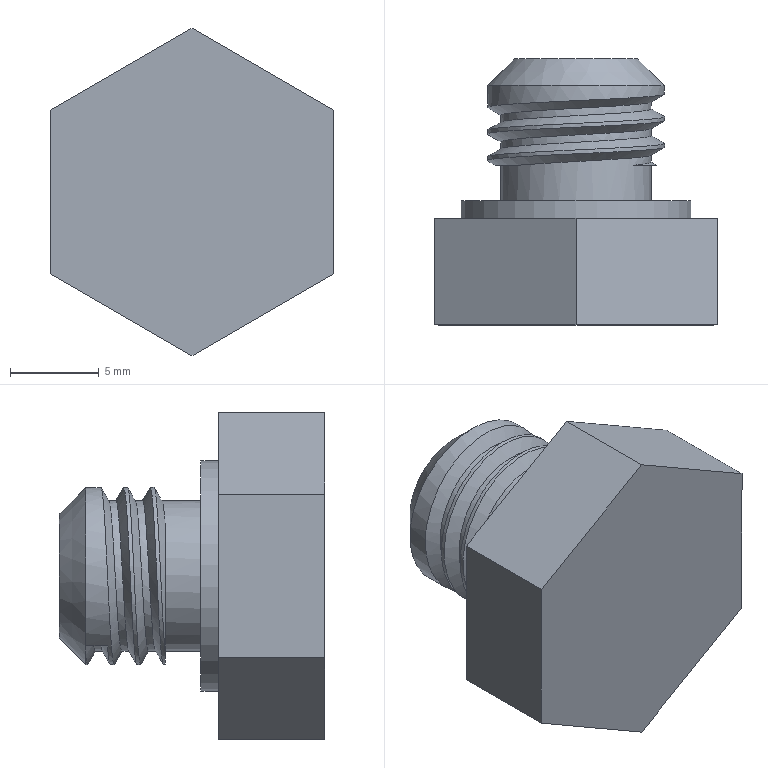Part | NX | features DATUM_CSYS 3, SKETCH 2, EXTRUDE 1, SWP104 1, THREADS 1 | 1 solid | 21 faces | box 16 x 15 x 18.475 mm | volume 1967 mm3 | plane 12 | cylinder 6 | spline 2 | cone 1 | commonest cylinder face diameters 8.5 x4 10 x1 13 x1
STEP:
#1=CARTESIAN_POINT('',(8.,0.,4.619));
#2=VERTEX_POINT('',#1);
#3=CARTESIAN_POINT('',(0.,0.,9.238));
#4=VERTEX_POINT('',#3);
#5=CARTESIAN_POINT('',(8.,0.,4.619));
#6=DIRECTION('',(-0.866,0.,0.5));
#7=VECTOR('',#6,1000.);
#8=LINE('',#5,#7);
#9=EDGE_CURVE('',#2,#4,#8,.T.);
#10=ORIENTED_EDGE('',*,*,#9,.T.);
#11=CARTESIAN_POINT('',(0.,-6.,9.238));
#12=VERTEX_POINT('',#11);
#13=CARTESIAN_POINT('',(0.,-6.,9.238));
#14=DIRECTION('',(0.,1.,0.));
#15=VECTOR('',#14,1000.);
#16=LINE('',#13,#15);
#17=EDGE_CURVE('',#12,#4,#16,.T.);
#18=ORIENTED_EDGE('',*,*,#17,.F.);
#19=CARTESIAN_POINT('',(8.,-6.,4.619));
#20=VERTEX_POINT('',#19);
#21=CARTESIAN_POINT('',(8.,-6.,4.619));
#22=DIRECTION('',(-0.866,0.,0.5));
#23=VECTOR('',#22,1000.);
#24=LINE('',#21,#23);
#25=EDGE_CURVE('',#20,#12,#24,.T.);
#26=ORIENTED_EDGE('',*,*,#25,.F.);
#27=CARTESIAN_POINT('',(8.,-6.,4.619));
#28=DIRECTION('',(0.,1.,0.));
#29=VECTOR('',#28,1000.);
#30=LINE('',#27,#29);
#31=EDGE_CURVE('',#20,#2,#30,.T.);
#32=ORIENTED_EDGE('',*,*,#31,.T.);
#33=EDGE_LOOP('',(#10,#18,#26,#32));
#34=FACE_BOUND('',#33,.T.);
#35=CARTESIAN_POINT('',(8.,-6.,4.619));
#36=DIRECTION('',(-0.5,0.,-0.866));
#37=DIRECTION('',(-0.866,0.,0.5));
#38=AXIS2_PLACEMENT_3D('',#35,#36,#37);
#39=PLANE('',#38);
#40=ADVANCED_FACE('',(#34),#39,.F.);
#41=CARTESIAN_POINT('',(-8.,0.,4.619));
#42=VERTEX_POINT('',#41);
#43=CARTESIAN_POINT('',(0.,0.,9.238));
#44=DIRECTION('',(-0.866,0.,-0.5));
#45=VECTOR('',#44,1000.);
#46=LINE('',#43,#45);
#47=EDGE_CURVE('',#4,#42,#46,.T.);
#48=ORIENTED_EDGE('',*,*,#47,.T.);
#49=CARTESIAN_POINT('',(-8.,-6.,4.619));
#50=VERTEX_POINT('',#49);
#51=CARTESIAN_POINT('',(-8.,-6.,4.619));
#52=DIRECTION('',(0.,1.,0.));
#53=VECTOR('',#52,1000.);
#54=LINE('',#51,#53);
#55=EDGE_CURVE('',#50,#42,#54,.T.);
#56=ORIENTED_EDGE('',*,*,#55,.F.);
#57=CARTESIAN_POINT('',(0.,-6.,9.238));
#58=DIRECTION('',(-0.866,0.,-0.5));
#59=VECTOR('',#58,1000.);
#60=LINE('',#57,#59);
#61=EDGE_CURVE('',#12,#50,#60,.T.);
#62=ORIENTED_EDGE('',*,*,#61,.F.);
#63=ORIENTED_EDGE('',*,*,#17,.T.);
#64=EDGE_LOOP('',(#48,#56,#62,#63));
#65=FACE_BOUND('',#64,.T.);
#66=CARTESIAN_POINT('',(0.,-6.,9.238));
#67=DIRECTION('',(0.5,0.,-0.866));
#68=DIRECTION('',(-0.866,0.,-0.5));
#69=AXIS2_PLACEMENT_3D('',#66,#67,#68);
#70=PLANE('',#69);
#71=ADVANCED_FACE('',(#65),#70,.F.);
#72=CARTESIAN_POINT('',(-8.,0.,-4.619));
#73=VERTEX_POINT('',#72);
#74=CARTESIAN_POINT('',(-8.,0.,4.619));
#75=DIRECTION('',(0.,0.,-1.));
#76=VECTOR('',#75,1000.);
#77=LINE('',#74,#76);
#78=EDGE_CURVE('',#42,#73,#77,.T.);
#79=ORIENTED_EDGE('',*,*,#78,.T.);
#80=CARTESIAN_POINT('',(-8.,-6.,-4.619));
#81=VERTEX_POINT('',#80);
#82=CARTESIAN_POINT('',(-8.,-6.,-4.619));
#83=DIRECTION('',(0.,1.,0.));
#84=VECTOR('',#83,1000.);
#85=LINE('',#82,#84);
#86=EDGE_CURVE('',#81,#73,#85,.T.);
#87=ORIENTED_EDGE('',*,*,#86,.F.);
#88=CARTESIAN_POINT('',(-8.,-6.,4.619));
#89=DIRECTION('',(0.,0.,-1.));
#90=VECTOR('',#89,1000.);
#91=LINE('',#88,#90);
#92=EDGE_CURVE('',#50,#81,#91,.T.);
#93=ORIENTED_EDGE('',*,*,#92,.F.);
#94=ORIENTED_EDGE('',*,*,#55,.T.);
#95=EDGE_LOOP('',(#79,#87,#93,#94));
#96=FACE_BOUND('',#95,.T.);
#97=CARTESIAN_POINT('',(-8.,-6.,4.619));
#98=DIRECTION('',(1.,0.,0.));
#99=DIRECTION('',(0.,0.,-1.));
#100=AXIS2_PLACEMENT_3D('',#97,#98,#99);
#101=PLANE('',#100);
#102=ADVANCED_FACE('',(#96),#101,.F.);
#103=CARTESIAN_POINT('',(0.,0.,-9.238));
#104=VERTEX_POINT('',#103);
#105=CARTESIAN_POINT('',(-8.,0.,-4.619));
#106=DIRECTION('',(0.866,0.,-0.5));
#107=VECTOR('',#106,1000.);
#108=LINE('',#105,#107);
#109=EDGE_CURVE('',#73,#104,#108,.T.);
#110=ORIENTED_EDGE('',*,*,#109,.T.);
#111=CARTESIAN_POINT('',(0.,-6.,-9.238));
#112=VERTEX_POINT('',#111);
#113=CARTESIAN_POINT('',(0.,-6.,-9.238));
#114=DIRECTION('',(0.,1.,0.));
#115=VECTOR('',#114,1000.);
#116=LINE('',#113,#115);
#117=EDGE_CURVE('',#112,#104,#116,.T.);
#118=ORIENTED_EDGE('',*,*,#117,.F.);
#119=CARTESIAN_POINT('',(-8.,-6.,-4.619));
#120=DIRECTION('',(0.866,0.,-0.5));
#121=VECTOR('',#120,1000.);
#122=LINE('',#119,#121);
#123=EDGE_CURVE('',#81,#112,#122,.T.);
#124=ORIENTED_EDGE('',*,*,#123,.F.);
#125=ORIENTED_EDGE('',*,*,#86,.T.);
#126=EDGE_LOOP('',(#110,#118,#124,#125));
#127=FACE_BOUND('',#126,.T.);
#128=CARTESIAN_POINT('',(-8.,-6.,-4.619));
#129=DIRECTION('',(0.5,0.,0.866));
#130=DIRECTION('',(0.866,0.,-0.5));
#131=AXIS2_PLACEMENT_3D('',#128,#129,#130);
#132=PLANE('',#131);
#133=ADVANCED_FACE('',(#127),#132,.F.);
#134=CARTESIAN_POINT('',(8.,0.,-4.619));
#135=VERTEX_POINT('',#134);
#136=CARTESIAN_POINT('',(0.,0.,-9.238));
#137=DIRECTION('',(0.866,0.,0.5));
#138=VECTOR('',#137,1000.);
#139=LINE('',#136,#138);
#140=EDGE_CURVE('',#104,#135,#139,.T.);
#141=ORIENTED_EDGE('',*,*,#140,.T.);
#142=CARTESIAN_POINT('',(8.,-6.,-4.619));
#143=VERTEX_POINT('',#142);
#144=CARTESIAN_POINT('',(8.,-6.,-4.619));
#145=DIRECTION('',(0.,1.,0.));
#146=VECTOR('',#145,1000.);
#147=LINE('',#144,#146);
#148=EDGE_CURVE('',#143,#135,#147,.T.);
#149=ORIENTED_EDGE('',*,*,#148,.F.);
#150=CARTESIAN_POINT('',(0.,-6.,-9.238));
#151=DIRECTION('',(0.866,0.,0.5));
#152=VECTOR('',#151,1000.);
#153=LINE('',#150,#152);
#154=EDGE_CURVE('',#112,#143,#153,.T.);
#155=ORIENTED_EDGE('',*,*,#154,.F.);
#156=ORIENTED_EDGE('',*,*,#117,.T.);
#157=EDGE_LOOP('',(#141,#149,#155,#156));
#158=FACE_BOUND('',#157,.T.);
#159=CARTESIAN_POINT('',(0.,-6.,-9.238));
#160=DIRECTION('',(-0.5,0.,0.866));
#161=DIRECTION('',(0.866,0.,0.5));
#162=AXIS2_PLACEMENT_3D('',#159,#160,#161);
#163=PLANE('',#162);
#164=ADVANCED_FACE('',(#158),#163,.F.);
#165=CARTESIAN_POINT('',(8.,0.,-4.619));
#166=DIRECTION('',(0.,0.,1.));
#167=VECTOR('',#166,1000.);
#168=LINE('',#165,#167);
#169=EDGE_CURVE('',#135,#2,#168,.T.);
#170=ORIENTED_EDGE('',*,*,#169,.T.);
#171=ORIENTED_EDGE('',*,*,#31,.F.);
#172=CARTESIAN_POINT('',(8.,-6.,-4.619));
#173=DIRECTION('',(0.,0.,1.));
#174=VECTOR('',#173,1000.);
#175=LINE('',#172,#174);
#176=EDGE_CURVE('',#143,#20,#175,.T.);
#177=ORIENTED_EDGE('',*,*,#176,.F.);
#178=ORIENTED_EDGE('',*,*,#148,.T.);
#179=EDGE_LOOP('',(#170,#171,#177,#178));
#180=FACE_BOUND('',#179,.T.);
#181=CARTESIAN_POINT('',(8.,-6.,-4.619));
#182=DIRECTION('',(-1.,0.,0.));
#183=DIRECTION('',(0.,0.,1.));
#184=AXIS2_PLACEMENT_3D('',#181,#182,#183);
#185=PLANE('',#184);
#186=ADVANCED_FACE('',(#180),#185,.F.);
#187=ORIENTED_EDGE('',*,*,#25,.T.);
#188=ORIENTED_EDGE('',*,*,#61,.T.);
#189=ORIENTED_EDGE('',*,*,#92,.T.);
#190=ORIENTED_EDGE('',*,*,#123,.T.);
#191=ORIENTED_EDGE('',*,*,#154,.T.);
#192=ORIENTED_EDGE('',*,*,#176,.T.);
#193=EDGE_LOOP('',(#187,#188,#189,#190,#191,#192));
#194=FACE_BOUND('',#193,.T.);
#195=CARTESIAN_POINT('',(0.,-6.,0.));
#196=DIRECTION('',(0.,-1.,0.));
#197=DIRECTION('',(0.,0.,-1.));
#198=AXIS2_PLACEMENT_3D('',#195,#196,#197);
#199=PLANE('',#198);
#200=ADVANCED_FACE('',(#194),#199,.T.);
#201=CARTESIAN_POINT('',(0.,0.,-6.5));
#202=VERTEX_POINT('',#201);
#203=CARTESIAN_POINT('',(0.,0.,0.));
#204=DIRECTION('',(0.,-1.,0.));
#205=DIRECTION('',(0.,0.,-1.));
#206=AXIS2_PLACEMENT_3D('',#203,#204,#205);
#207=CIRCLE('',#206,6.5);
#208=EDGE_CURVE('',#202,#202,#207,.T.);
#209=ORIENTED_EDGE('',*,*,#208,.T.);
#210=EDGE_LOOP('',(#209));
#211=FACE_BOUND('',#210,.T.);
#212=ORIENTED_EDGE('',*,*,#9,.F.);
#213=ORIENTED_EDGE('',*,*,#169,.F.);
#214=ORIENTED_EDGE('',*,*,#140,.F.);
#215=ORIENTED_EDGE('',*,*,#109,.F.);
#216=ORIENTED_EDGE('',*,*,#78,.F.);
#217=ORIENTED_EDGE('',*,*,#47,.F.);
#218=EDGE_LOOP('',(#212,#213,#214,#215,#216,#217));
#219=FACE_BOUND('',#218,.T.);
#220=CARTESIAN_POINT('',(0.,0.,0.));
#221=DIRECTION('',(0.,-1.,0.));
#222=DIRECTION('',(0.,0.,-1.));
#223=AXIS2_PLACEMENT_3D('',#220,#221,#222);
#224=PLANE('',#223);
#225=ADVANCED_FACE('',(#211,#219),#224,.F.);
#226=CARTESIAN_POINT('',(-2.211,7.5,-4.485));
#227=VERTEX_POINT('',#226);
#228=CARTESIAN_POINT('',(-3.071,7.5,-3.945));
#229=VERTEX_POINT('',#228);
#230=CARTESIAN_POINT('',(0.,7.5,0.));
#231=DIRECTION('',(0.,-1.,0.));
#232=DIRECTION('',(0.,0.,-1.));
#233=AXIS2_PLACEMENT_3D('',#230,#231,#232);
#234=CIRCLE('',#233,5.);
#235=EDGE_CURVE('',#227,#229,#234,.T.);
#236=ORIENTED_EDGE('',*,*,#235,.T.);
#237=CARTESIAN_POINT('',(-3.071,6.267,-3.945));
#238=VERTEX_POINT('',#237);
#239=CARTESIAN_POINT('',(-3.071,0.,-3.945));
#240=DIRECTION('',(0.,-1.,0.));
#241=VECTOR('',#240,1000.);
#242=LINE('',#239,#241);
#243=EDGE_CURVE('',#229,#238,#242,.T.);
#244=ORIENTED_EDGE('',*,*,#243,.T.);
#245=CARTESIAN_POINT('',(2.211,3.,-4.485));
#246=VERTEX_POINT('',#245);
#247=CARTESIAN_POINT('',(-3.071,6.267,-3.945));
#248=CARTESIAN_POINT('',(-1.936,6.198,-4.829));
#249=CARTESIAN_POINT('',(1.08,6.063,-5.537));
#250=CARTESIAN_POINT('',(4.899,5.859,-2.814));
#251=CARTESIAN_POINT('',(5.337,5.655,1.848));
#252=CARTESIAN_POINT('',(2.102,5.45,5.241));
#253=CARTESIAN_POINT('',(-2.572,5.246,5.028));
#254=CARTESIAN_POINT('',(-5.484,5.042,1.351));
#255=CARTESIAN_POINT('',(-4.621,4.838,-3.247));
#256=CARTESIAN_POINT('',(-0.5735,4.634,-5.618));
#257=CARTESIAN_POINT('',(3.859,4.43,-4.123));
#258=CARTESIAN_POINT('',(5.644,4.225,0.2145));
#259=CARTESIAN_POINT('',(3.545,4.021,4.396));
#260=CARTESIAN_POINT('',(-0.9981,3.817,5.559));
#261=CARTESIAN_POINT('',(-4.847,3.613,2.897));
#262=CARTESIAN_POINT('',(-5.367,3.409,-1.763));
#263=CARTESIAN_POINT('',(-2.187,3.204,-5.202));
#264=CARTESIAN_POINT('',(0.9203,3.069,-5.121));
#265=CARTESIAN_POINT('',(2.211,3.,-4.485));
#266=B_SPLINE_CURVE_WITH_KNOTS('',3,(#247,#248,#249,#250,#251,#252,#253,#254,#255,#256,#257,#258,#259,#260,#261,#262,#263,#264,#265),.UNSPECIFIED.,.F.,.F.,(4,1,1,1,1,1,1,1,1,1,1,1,1,1,1,1,4),(0.,0.004261,0.008522,0.01278,0.01704,0.02131,0.02557,0.02983,0.03409,0.03835,0.04261,0.04687,0.05113,0.05539,0.05965,0.06392,0.06818),.UNSPECIFIED.);
#267=EDGE_CURVE('',#238,#246,#266,.T.);
#268=ORIENTED_EDGE('',*,*,#267,.T.);
#269=CARTESIAN_POINT('',(-2.211,3.,-4.485));
#270=VERTEX_POINT('',#269);
#271=CARTESIAN_POINT('',(0.,3.,0.));
#272=DIRECTION('',(0.,-1.,0.));
#273=DIRECTION('',(0.,0.,-1.));
#274=AXIS2_PLACEMENT_3D('',#271,#272,#273);
#275=CIRCLE('',#274,5.);
#276=EDGE_CURVE('',#270,#246,#275,.T.);
#277=ORIENTED_EDGE('',*,*,#276,.F.);
#278=CARTESIAN_POINT('',(-2.211,3.,-4.485));
#279=CARTESIAN_POINT('',(-3.1,3.048,-4.046));
#280=CARTESIAN_POINT('',(-4.582,3.14,-2.654));
#281=CARTESIAN_POINT('',(-5.288,3.281,0.3466));
#282=CARTESIAN_POINT('',(-4.201,3.422,3.226));
#283=CARTESIAN_POINT('',(-1.704,3.562,5.015));
#284=CARTESIAN_POINT('',(1.368,3.703,5.118));
#285=CARTESIAN_POINT('',(3.983,3.844,3.494));
#286=CARTESIAN_POINT('',(5.252,3.985,0.6902));
#287=CARTESIAN_POINT('',(4.752,4.125,-2.34));
#288=CARTESIAN_POINT('',(2.652,4.266,-4.586));
#289=CARTESIAN_POINT('',(-0.3453,4.406,-5.287));
#290=CARTESIAN_POINT('',(-3.225,4.547,-4.202));
#291=CARTESIAN_POINT('',(-5.015,4.687,-1.706));
#292=CARTESIAN_POINT('',(-5.118,4.828,1.367));
#293=CARTESIAN_POINT('',(-3.495,4.969,3.982));
#294=CARTESIAN_POINT('',(-0.6915,5.11,5.252));
#295=CARTESIAN_POINT('',(2.338,5.25,4.753));
#296=CARTESIAN_POINT('',(4.586,5.391,2.653));
#297=CARTESIAN_POINT('',(5.287,5.531,-0.3446));
#298=CARTESIAN_POINT('',(4.203,5.672,-3.224));
#299=CARTESIAN_POINT('',(1.708,5.812,-5.014));
#300=CARTESIAN_POINT('',(-1.367,5.953,-5.119));
#301=CARTESIAN_POINT('',(-3.982,6.094,-3.495));
#302=CARTESIAN_POINT('',(-5.251,6.234,-0.6931));
#303=CARTESIAN_POINT('',(-4.754,6.375,2.337));
#304=CARTESIAN_POINT('',(-2.654,6.516,4.586));
#305=CARTESIAN_POINT('',(0.3439,6.656,5.287));
#306=CARTESIAN_POINT('',(3.223,6.797,4.204));
#307=CARTESIAN_POINT('',(5.014,6.937,1.71));
#308=CARTESIAN_POINT('',(5.119,7.078,-1.366));
#309=CARTESIAN_POINT('',(3.496,7.218,-3.982));
#310=CARTESIAN_POINT('',(0.6934,7.36,-5.25));
#311=CARTESIAN_POINT('',(-1.322,7.452,-4.923));
#312=CARTESIAN_POINT('',(-2.211,7.5,-4.485));
#313=B_SPLINE_CURVE_WITH_KNOTS('',3,(#278,#279,#280,#281,#282,#283,#284,#285,#286,#287,#288,#289,#290,#291,#292,#293,#294,#295,#296,#297,#298,#299,#300,#301,#302,#303,#304,#305,#306,#307,#308,#309,#310,#311,#312),.UNSPECIFIED.,.F.,.F.,(4,1,1,1,1,1,1,1,1,1,1,1,1,1,1,1,1,1,1,1,1,1,1,1,1,1,1,1,1,1,1,1,4),(0.,0.002934,0.005869,0.008803,0.01174,0.01467,0.01761,0.02054,0.02348,0.02641,0.02934,0.03228,0.03521,0.03815,0.04108,0.04402,0.04695,0.04989,0.05282,0.05576,0.05869,0.06162,0.06456,0.06749,0.07043,0.07336,0.0763,0.07923,0.08217,0.0851,0.08803,0.09097,0.0939),.UNSPECIFIED.);
#314=EDGE_CURVE('',#270,#227,#313,.T.);
#315=ORIENTED_EDGE('',*,*,#314,.T.);
#316=EDGE_LOOP('',(#236,#244,#268,#277,#315));
#317=FACE_BOUND('',#316,.T.);
#318=CARTESIAN_POINT('',(0.,0.,0.));
#319=DIRECTION('',(0.,-1.,0.));
#320=DIRECTION('',(0.,0.,-1.));
#321=AXIS2_PLACEMENT_3D('',#318,#319,#320);
#322=CYLINDRICAL_SURFACE('',#321,5.);
#323=ADVANCED_FACE('',(#317),#322,.T.);
#324=ORIENTED_EDGE('',*,*,#276,.T.);
#325=CARTESIAN_POINT('',(3.248,3.,2.741));
#326=VERTEX_POINT('',#325);
#327=CARTESIAN_POINT('',(2.211,3.,-4.485));
#328=CARTESIAN_POINT('',(3.421,3.,-3.758));
#329=CARTESIAN_POINT('',(5.166,3.,-1.231));
#330=CARTESIAN_POINT('',(4.262,3.,1.752));
#331=CARTESIAN_POINT('',(3.248,3.,2.741));
#332=B_SPLINE_CURVE_WITH_KNOTS('',3,(#327,#328,#329,#330,#331),.UNSPECIFIED.,.F.,.F.,(4,1,4),(0.0001186,0.004308,0.008497),.UNSPECIFIED.);
#333=EDGE_CURVE('',#246,#326,#332,.T.);
#334=ORIENTED_EDGE('',*,*,#333,.T.);
#335=CARTESIAN_POINT('',(-3.248,3.,2.741));
#336=VERTEX_POINT('',#335);
#337=CARTESIAN_POINT('',(0.,3.,0.));
#338=DIRECTION('',(0.,-1.,0.));
#339=DIRECTION('',(0.,0.,-1.));
#340=AXIS2_PLACEMENT_3D('',#337,#338,#339);
#341=CIRCLE('',#340,4.25);
#342=EDGE_CURVE('',#336,#326,#341,.T.);
#343=ORIENTED_EDGE('',*,*,#342,.F.);
#344=CARTESIAN_POINT('',(-3.248,3.,2.741));
#345=CARTESIAN_POINT('',(-4.26,3.,1.753));
#346=CARTESIAN_POINT('',(-5.168,3.,-1.228));
#347=CARTESIAN_POINT('',(-3.42,3.,-3.758));
#348=CARTESIAN_POINT('',(-2.211,3.,-4.485));
#349=B_SPLINE_CURVE_WITH_KNOTS('',3,(#344,#345,#346,#347,#348),.UNSPECIFIED.,.F.,.F.,(4,1,4),(0.00004919,0.004257,0.008466),.UNSPECIFIED.);
#350=EDGE_CURVE('',#336,#270,#349,.T.);
#351=ORIENTED_EDGE('',*,*,#350,.T.);
#352=EDGE_LOOP('',(#324,#334,#343,#351));
#353=FACE_BOUND('',#352,.T.);
#354=CARTESIAN_POINT('',(0.,3.,5.));
#355=DIRECTION('',(0.,1.,0.));
#356=DIRECTION('',(0.,0.,1.));
#357=AXIS2_PLACEMENT_3D('',#354,#355,#356);
#358=PLANE('',#357);
#359=ADVANCED_FACE('',(#353),#358,.F.);
#360=CARTESIAN_POINT('',(0.,1.,-4.25));
#361=VERTEX_POINT('',#360);
#362=CARTESIAN_POINT('',(0.,1.,0.));
#363=DIRECTION('',(0.,-1.,0.));
#364=DIRECTION('',(0.,0.,-1.));
#365=AXIS2_PLACEMENT_3D('',#362,#363,#364);
#366=CIRCLE('',#365,4.25);
#367=EDGE_CURVE('',#361,#361,#366,.T.);
#368=ORIENTED_EDGE('',*,*,#367,.F.);
#369=EDGE_LOOP('',(#368));
#370=FACE_BOUND('',#369,.T.);
#371=ORIENTED_EDGE('',*,*,#342,.T.);
#372=CARTESIAN_POINT('',(-2.611,6.7,-3.354));
#373=VERTEX_POINT('',#372);
#374=CARTESIAN_POINT('',(-2.611,6.7,-3.354));
#375=CARTESIAN_POINT('',(-1.518,6.622,-4.205));
#376=CARTESIAN_POINT('',(1.501,6.469,-4.728));
#377=CARTESIAN_POINT('',(4.755,6.238,-1.443));
#378=CARTESIAN_POINT('',(3.881,6.006,3.102));
#379=CARTESIAN_POINT('',(-0.3584,5.775,4.955));
#380=CARTESIAN_POINT('',(-4.288,5.544,2.51));
#381=CARTESIAN_POINT('',(-4.497,5.313,-2.113));
#382=CARTESIAN_POINT('',(-0.8052,5.081,-4.902));
#383=CARTESIAN_POINT('',(3.584,4.85,-3.44));
#384=CARTESIAN_POINT('',(4.865,4.619,1.003));
#385=CARTESIAN_POINT('',(1.93,4.388,4.578));
#386=CARTESIAN_POINT('',(-2.68,4.156,4.184));
#387=CARTESIAN_POINT('',(-4.966,3.925,0.1601));
#388=CARTESIAN_POINT('',(-2.944,3.694,-4.002));
#389=CARTESIAN_POINT('',(1.634,3.463,-4.694));
#390=CARTESIAN_POINT('',(4.786,3.231,-1.306));
#391=CARTESIAN_POINT('',(4.14,3.077,1.685));
#392=CARTESIAN_POINT('',(3.248,3.,2.741));
#393=B_SPLINE_CURVE_WITH_KNOTS('',3,(#374,#375,#376,#377,#378,#379,#380,#381,#382,#383,#384,#385,#386,#387,#388,#389,#390,#391,#392),.UNSPECIFIED.,.F.,.F.,(4,1,1,1,1,1,1,1,1,1,1,1,1,1,1,1,4),(0.,0.004122,0.008243,0.01236,0.01649,0.02061,0.02473,0.02885,0.03297,0.03709,0.04122,0.04534,0.04946,0.05358,0.0577,0.06182,0.06595),.UNSPECIFIED.);
#394=EDGE_CURVE('',#373,#326,#393,.T.);
#395=ORIENTED_EDGE('',*,*,#394,.F.);
#396=CARTESIAN_POINT('',(-2.611,7.116,-3.354));
#397=VERTEX_POINT('',#396);
#398=CARTESIAN_POINT('',(-2.611,2.25,-3.354));
#399=DIRECTION('',(0.,1.,0.));
#400=VECTOR('',#399,1000.);
#401=LINE('',#398,#400);
#402=EDGE_CURVE('',#397,#373,#401,.F.);
#403=ORIENTED_EDGE('',*,*,#402,.F.);
#404=CARTESIAN_POINT('',(-3.248,3.,2.741));
#405=CARTESIAN_POINT('',(-2.259,3.086,3.912));
#406=CARTESIAN_POINT('',(1.06,3.258,5.037));
#407=CARTESIAN_POINT('',(4.948,3.515,1.451));
#408=CARTESIAN_POINT('',(3.62,3.772,-3.669));
#409=CARTESIAN_POINT('',(-1.514,4.029,-4.926));
#410=CARTESIAN_POINT('',(-5.057,4.286,-1.));
#411=CARTESIAN_POINT('',(-3.274,4.543,3.982));
#412=CARTESIAN_POINT('',(1.957,4.801,4.768));
#413=CARTESIAN_POINT('',(5.126,5.058,0.5354));
#414=CARTESIAN_POINT('',(2.901,5.315,-4.26));
#415=CARTESIAN_POINT('',(-2.377,5.572,-4.573));
#416=CARTESIAN_POINT('',(-5.155,5.829,-0.07114));
#417=CARTESIAN_POINT('',(-2.501,6.087,4.507));
#418=CARTESIAN_POINT('',(2.783,6.344,4.338));
#419=CARTESIAN_POINT('',(5.141,6.601,-0.3979));
#420=CARTESIAN_POINT('',(2.078,6.858,-4.706));
#421=CARTESIAN_POINT('',(-1.395,7.029,-4.3));
#422=CARTESIAN_POINT('',(-2.611,7.116,-3.354));
#423=B_SPLINE_CURVE_WITH_KNOTS('',3,(#404,#405,#406,#407,#408,#409,#410,#411,#412,#413,#414,#415,#416,#417,#418,#419,#420,#421,#422),.UNSPECIFIED.,.F.,.F.,(4,1,1,1,1,1,1,1,1,1,1,1,1,1,1,1,4),(0.009664,0.01425,0.01883,0.02342,0.028,0.03259,0.03717,0.04175,0.04634,0.05092,0.05551,0.06009,0.06468,0.06926,0.07384,0.07843,0.08301),.UNSPECIFIED.);
#424=EDGE_CURVE('',#336,#397,#423,.T.);
#425=ORIENTED_EDGE('',*,*,#424,.F.);
#426=EDGE_LOOP('',(#371,#395,#403,#425));
#427=FACE_BOUND('',#426,.T.);
#428=CARTESIAN_POINT('',(0.,0.,0.));
#429=DIRECTION('',(0.,-1.,0.));
#430=DIRECTION('',(0.,0.,-1.));
#431=AXIS2_PLACEMENT_3D('',#428,#429,#430);
#432=CYLINDRICAL_SURFACE('',#431,4.25);
#433=ADVANCED_FACE('',(#370,#427),#432,.T.);
#434=CARTESIAN_POINT('',(0.,1.,-6.5));
#435=VERTEX_POINT('',#434);
#436=CARTESIAN_POINT('',(0.,1.,0.));
#437=DIRECTION('',(0.,-1.,0.));
#438=DIRECTION('',(0.,0.,-1.));
#439=AXIS2_PLACEMENT_3D('',#436,#437,#438);
#440=CIRCLE('',#439,6.5);
#441=EDGE_CURVE('',#435,#435,#440,.T.);
#442=ORIENTED_EDGE('',*,*,#441,.F.);
#443=EDGE_LOOP('',(#442));
#444=FACE_BOUND('',#443,.T.);
#445=ORIENTED_EDGE('',*,*,#367,.T.);
#446=EDGE_LOOP('',(#445));
#447=FACE_BOUND('',#446,.T.);
#448=CARTESIAN_POINT('',(0.,1.,4.25));
#449=DIRECTION('',(0.,-1.,0.));
#450=DIRECTION('',(0.,0.,-1.));
#451=AXIS2_PLACEMENT_3D('',#448,#449,#450);
#452=PLANE('',#451);
#453=ADVANCED_FACE('',(#444,#447),#452,.F.);
#454=ORIENTED_EDGE('',*,*,#208,.F.);
#455=EDGE_LOOP('',(#454));
#456=FACE_BOUND('',#455,.T.);
#457=ORIENTED_EDGE('',*,*,#441,.T.);
#458=EDGE_LOOP('',(#457));
#459=FACE_BOUND('',#458,.T.);
#460=CARTESIAN_POINT('',(0.,0.,0.));
#461=DIRECTION('',(0.,-1.,0.));
#462=DIRECTION('',(0.,0.,-1.));
#463=AXIS2_PLACEMENT_3D('',#460,#461,#462);
#464=CYLINDRICAL_SURFACE('',#463,6.5);
#465=ADVANCED_FACE('',(#456,#459),#464,.T.);
#466=CARTESIAN_POINT('',(0.,9.,-3.5));
#467=VERTEX_POINT('',#466);
#468=CARTESIAN_POINT('',(0.,9.,0.));
#469=DIRECTION('',(0.,-1.,0.));
#470=DIRECTION('',(0.,0.,-1.));
#471=AXIS2_PLACEMENT_3D('',#468,#469,#470);
#472=CIRCLE('',#471,3.5);
#473=EDGE_CURVE('',#467,#467,#472,.T.);
#474=ORIENTED_EDGE('',*,*,#473,.F.);
#475=EDGE_LOOP('',(#474));
#476=FACE_BOUND('',#475,.T.);
#477=CARTESIAN_POINT('',(0.,9.,0.));
#478=DIRECTION('',(0.,-1.,0.));
#479=DIRECTION('',(0.,0.,-1.));
#480=AXIS2_PLACEMENT_3D('',#477,#478,#479);
#481=PLANE('',#480);
#482=ADVANCED_FACE('',(#476),#481,.F.);
#483=CARTESIAN_POINT('',(-3.053,7.531,-3.921));
#484=VERTEX_POINT('',#483);
#485=CARTESIAN_POINT('',(-2.211,7.5,-4.485));
#486=CARTESIAN_POINT('',(-2.511,7.51,-4.325));
#487=CARTESIAN_POINT('',(-2.791,7.521,-4.138));
#488=CARTESIAN_POINT('',(-3.053,7.531,-3.921));
#489=B_SPLINE_CURVE_WITH_KNOTS('',3,(#485,#486,#487,#488),.UNSPECIFIED.,.F.,.F.,(4,4),(0.,0.001013),.UNSPECIFIED.);
#490=EDGE_CURVE('',#227,#484,#489,.T.);
#491=ORIENTED_EDGE('',*,*,#490,.T.);
#492=CARTESIAN_POINT('',(0.,12.5,0.));
#493=DIRECTION('',(-0.4344,-0.7071,-0.558));
#494=VECTOR('',#493,1000.);
#495=LINE('',#492,#494);
#496=EDGE_CURVE('',#484,#229,#495,.T.);
#497=ORIENTED_EDGE('',*,*,#496,.T.);
#498=ORIENTED_EDGE('',*,*,#235,.F.);
#499=EDGE_LOOP('',(#491,#497,#498));
#500=FACE_BOUND('',#499,.T.);
#501=ORIENTED_EDGE('',*,*,#473,.T.);
#502=EDGE_LOOP('',(#501));
#503=FACE_BOUND('',#502,.T.);
#504=CARTESIAN_POINT('',(0.,9.,0.));
#505=DIRECTION('',(0.,-1.,0.));
#506=DIRECTION('',(0.,0.,-1.));
#507=AXIS2_PLACEMENT_3D('',#504,#505,#506);
#508=CONICAL_SURFACE('',#507,3.5,0.7854);
#509=ADVANCED_FACE('',(#500,#503),#508,.T.);
#510=ORIENTED_EDGE('',*,*,#496,.F.);
#511=CARTESIAN_POINT('',(-2.459,6.973,-3.158));
#512=CARTESIAN_POINT('',(-3.077,7.554,-3.953));
#513=B_SPLINE_CURVE_WITH_KNOTS('',1,(#511,#512),.UNSPECIFIED.,.F.,.F.,(2,2),(0.,1.),.PIECEWISE_BEZIER_KNOTS.);
#514=EDGE_CURVE('',#397,#484,#513,.T.);
#515=ORIENTED_EDGE('',*,*,#514,.F.);
#516=ORIENTED_EDGE('',*,*,#402,.T.);
#517=CARTESIAN_POINT('',(-3.077,6.262,-3.953));
#518=CARTESIAN_POINT('',(-2.459,6.843,-3.158));
#519=B_SPLINE_CURVE_WITH_KNOTS('',1,(#517,#518),.UNSPECIFIED.,.F.,.F.,(2,2),(0.,1.),.PIECEWISE_BEZIER_KNOTS.);
#520=EDGE_CURVE('',#238,#373,#519,.T.);
#521=ORIENTED_EDGE('',*,*,#520,.F.);
#522=ORIENTED_EDGE('',*,*,#243,.F.);
#523=EDGE_LOOP('',(#510,#515,#516,#521,#522));
#524=FACE_BOUND('',#523,.T.);
#525=CARTESIAN_POINT('',(-3.077,6.908,-3.953));
#526=DIRECTION('',(-0.7891,0.,0.6143));
#527=DIRECTION('',(0.6143,0.,0.7891));
#528=AXIS2_PLACEMENT_3D('',#525,#526,#527);
#529=PLANE('',#528);
#530=ADVANCED_FACE('',(#524),#529,.F.);
#531=ORIENTED_EDGE('',*,*,#520,.T.);
#532=ORIENTED_EDGE('',*,*,#394,.T.);
#533=ORIENTED_EDGE('',*,*,#333,.F.);
#534=ORIENTED_EDGE('',*,*,#267,.F.);
#535=EDGE_LOOP('',(#531,#532,#533,#534));
#536=FACE_BOUND('',#535,.T.);
#537=CARTESIAN_POINT('',(3.508,2.542,3.57));
#538=CARTESIAN_POINT('',(3.519,2.543,3.559));
#539=CARTESIAN_POINT('',(3.994,2.575,3.088));
#540=CARTESIAN_POINT('',(4.744,2.638,1.965));
#541=CARTESIAN_POINT('',(5.135,2.732,0.));
#542=CARTESIAN_POINT('',(4.744,2.825,-1.965));
#543=CARTESIAN_POINT('',(3.631,2.919,-3.631));
#544=CARTESIAN_POINT('',(1.965,3.013,-4.744));
#545=CARTESIAN_POINT('',(0.,3.107,-5.135));
#546=CARTESIAN_POINT('',(-1.965,3.2,-4.744));
#547=CARTESIAN_POINT('',(-3.631,3.294,-3.631));
#548=CARTESIAN_POINT('',(-4.744,3.388,-1.965));
#549=CARTESIAN_POINT('',(-5.135,3.482,0.));
#550=CARTESIAN_POINT('',(-4.744,3.575,1.965));
#551=CARTESIAN_POINT('',(-3.631,3.669,3.631));
#552=CARTESIAN_POINT('',(-1.965,3.763,4.744));
#553=CARTESIAN_POINT('',(0.,3.857,5.135));
#554=CARTESIAN_POINT('',(1.965,3.95,4.744));
#555=CARTESIAN_POINT('',(3.631,4.044,3.631));
#556=CARTESIAN_POINT('',(4.744,4.138,1.965));
#557=CARTESIAN_POINT('',(5.135,4.232,0.));
#558=CARTESIAN_POINT('',(4.744,4.325,-1.965));
#559=CARTESIAN_POINT('',(3.631,4.419,-3.631));
#560=CARTESIAN_POINT('',(1.965,4.513,-4.744));
#561=CARTESIAN_POINT('',(0.,4.607,-5.135));
#562=CARTESIAN_POINT('',(-1.965,4.7,-4.744));
#563=CARTESIAN_POINT('',(-3.631,4.794,-3.631));
#564=CARTESIAN_POINT('',(-4.744,4.888,-1.965));
#565=CARTESIAN_POINT('',(-5.135,4.982,0.));
#566=CARTESIAN_POINT('',(-4.744,5.075,1.965));
#567=CARTESIAN_POINT('',(-3.631,5.169,3.631));
#568=CARTESIAN_POINT('',(-1.965,5.263,4.744));
#569=CARTESIAN_POINT('',(0.,5.357,5.135));
#570=CARTESIAN_POINT('',(1.965,5.45,4.744));
#571=CARTESIAN_POINT('',(3.631,5.544,3.631));
#572=CARTESIAN_POINT('',(4.744,5.638,1.965));
#573=CARTESIAN_POINT('',(5.135,5.732,0.));
#574=CARTESIAN_POINT('',(4.744,5.825,-1.965));
#575=CARTESIAN_POINT('',(3.631,5.919,-3.631));
#576=CARTESIAN_POINT('',(1.965,6.013,-4.744));
#577=CARTESIAN_POINT('',(0.,6.107,-5.135));
#578=CARTESIAN_POINT('',(-1.758,6.19,-4.785));
#579=CARTESIAN_POINT('',(-2.72,6.243,-4.224));
#580=CARTESIAN_POINT('',(-3.074,6.264,-3.949));
#581=CARTESIAN_POINT('',(2.976,2.981,3.028));
#582=CARTESIAN_POINT('',(2.985,2.981,3.019));
#583=CARTESIAN_POINT('',(3.388,3.013,2.619));
#584=CARTESIAN_POINT('',(4.024,3.076,1.667));
#585=CARTESIAN_POINT('',(4.356,3.17,0.));
#586=CARTESIAN_POINT('',(4.024,3.264,-1.667));
#587=CARTESIAN_POINT('',(3.08,3.358,-3.08));
#588=CARTESIAN_POINT('',(1.667,3.451,-4.024));
#589=CARTESIAN_POINT('',(0.,3.545,-4.356));
#590=CARTESIAN_POINT('',(-1.667,3.639,-4.024));
#591=CARTESIAN_POINT('',(-3.08,3.733,-3.08));
#592=CARTESIAN_POINT('',(-4.024,3.826,-1.667));
#593=CARTESIAN_POINT('',(-4.356,3.92,0.));
#594=CARTESIAN_POINT('',(-4.024,4.014,1.667));
#595=CARTESIAN_POINT('',(-3.08,4.108,3.08));
#596=CARTESIAN_POINT('',(-1.667,4.201,4.024));
#597=CARTESIAN_POINT('',(0.,4.295,4.356));
#598=CARTESIAN_POINT('',(1.667,4.389,4.024));
#599=CARTESIAN_POINT('',(3.08,4.483,3.08));
#600=CARTESIAN_POINT('',(4.024,4.576,1.667));
#601=CARTESIAN_POINT('',(4.356,4.67,0.));
#602=CARTESIAN_POINT('',(4.024,4.764,-1.667));
#603=CARTESIAN_POINT('',(3.08,4.858,-3.08));
#604=CARTESIAN_POINT('',(1.667,4.951,-4.024));
#605=CARTESIAN_POINT('',(0.,5.045,-4.356));
#606=CARTESIAN_POINT('',(-1.667,5.139,-4.024));
#607=CARTESIAN_POINT('',(-3.08,5.233,-3.08));
#608=CARTESIAN_POINT('',(-4.024,5.326,-1.667));
#609=CARTESIAN_POINT('',(-4.356,5.42,0.));
#610=CARTESIAN_POINT('',(-4.024,5.514,1.667));
#611=CARTESIAN_POINT('',(-3.08,5.608,3.08));
#612=CARTESIAN_POINT('',(-1.667,5.701,4.024));
#613=CARTESIAN_POINT('',(0.,5.795,4.356));
#614=CARTESIAN_POINT('',(1.667,5.889,4.024));
#615=CARTESIAN_POINT('',(3.08,5.983,3.08));
#616=CARTESIAN_POINT('',(4.024,6.076,1.667));
#617=CARTESIAN_POINT('',(4.356,6.17,0.));
#618=CARTESIAN_POINT('',(4.024,6.264,-1.667));
#619=CARTESIAN_POINT('',(3.08,6.358,-3.08));
#620=CARTESIAN_POINT('',(1.667,6.451,-4.024));
#621=CARTESIAN_POINT('',(0.,6.545,-4.356));
#622=CARTESIAN_POINT('',(-1.492,6.629,-4.059));
#623=CARTESIAN_POINT('',(-2.308,6.682,-3.583));
#624=CARTESIAN_POINT('',(-2.608,6.703,-3.35));
#625=B_SPLINE_SURFACE_WITH_KNOTS('',1,3,((#537,#538,#539,#540,#541,#542,#543,#544,#545,#546,#547,#548,#549,#550,#551,#552,#553,#554,#555,#556,#557,#558,#559,#560,#561,#562,#563,#564,#565,#566,#567,#568,#569,#570,#571,#572,#573,#574,#575,#576,#577,#578,#579,#580),(#581,#582,#583,#584,#585,#586,#587,#588,#589,#590,#591,#592,#593,#594,#595,#596,#597,#598,#599,#600,#601,#602,#603,#604,#605,#606,#607,#608,#609,#610,#611,#612,#613,#614,#615,#616,#617,#618,#619,#620,#621,#622,#623,#624)),.RULED_SURF.,.F.,.F.,.F.,(2,2),(4,1,1,1,1,1,1,1,1,1,1,1,1,1,1,1,1,1,1,1,1,1,1,1,1,1,1,1,1,1,1,1,1,1,1,1,1,1,1,1,1,4),(0.005015,0.7593),(0.2008,0.2013,0.2214,0.2415,0.2617,0.2818,0.3019,0.322,0.3422,0.3623,0.3824,0.4025,0.4227,0.4428,0.4629,0.483,0.5032,0.5233,0.5434,0.5636,0.5837,0.6038,0.6239,0.6441,0.6642,0.6843,0.7044,0.7246,0.7447,0.7648,0.785,0.8051,0.8252,0.8453,0.8655,0.8856,0.9057,0.9258,0.946,0.9661,0.9862,1.),.UNSPECIFIED.);
#626=ADVANCED_FACE('',(#536),#625,.F.);
#627=ORIENTED_EDGE('',*,*,#424,.T.);
#628=ORIENTED_EDGE('',*,*,#514,.T.);
#629=ORIENTED_EDGE('',*,*,#490,.F.);
#630=ORIENTED_EDGE('',*,*,#314,.F.);
#631=ORIENTED_EDGE('',*,*,#350,.F.);
#632=EDGE_LOOP('',(#627,#628,#629,#630,#631));
#633=FACE_BOUND('',#632,.T.);
#634=CARTESIAN_POINT('',(-1.431,2.537,-3.997));
#635=CARTESIAN_POINT('',(-1.496,2.541,-3.974));
#636=CARTESIAN_POINT('',(-2.079,2.576,-3.749));
#637=CARTESIAN_POINT('',(-3.08,2.642,-3.08));
#638=CARTESIAN_POINT('',(-4.024,2.736,-1.667));
#639=CARTESIAN_POINT('',(-4.356,2.83,0.));
#640=CARTESIAN_POINT('',(-4.024,2.924,1.667));
#641=CARTESIAN_POINT('',(-3.08,3.017,3.08));
#642=CARTESIAN_POINT('',(-1.667,3.111,4.024));
#643=CARTESIAN_POINT('',(0.,3.205,4.356));
#644=CARTESIAN_POINT('',(1.667,3.299,4.024));
#645=CARTESIAN_POINT('',(3.08,3.392,3.08));
#646=CARTESIAN_POINT('',(4.024,3.486,1.667));
#647=CARTESIAN_POINT('',(4.356,3.58,0.));
#648=CARTESIAN_POINT('',(4.024,3.674,-1.667));
#649=CARTESIAN_POINT('',(3.08,3.767,-3.08));
#650=CARTESIAN_POINT('',(1.667,3.861,-4.024));
#651=CARTESIAN_POINT('',(0.,3.955,-4.356));
#652=CARTESIAN_POINT('',(-1.667,4.049,-4.024));
#653=CARTESIAN_POINT('',(-3.08,4.142,-3.08));
#654=CARTESIAN_POINT('',(-4.024,4.236,-1.667));
#655=CARTESIAN_POINT('',(-4.356,4.33,0.));
#656=CARTESIAN_POINT('',(-4.024,4.424,1.667));
#657=CARTESIAN_POINT('',(-3.08,4.517,3.08));
#658=CARTESIAN_POINT('',(-1.667,4.611,4.024));
#659=CARTESIAN_POINT('',(0.,4.705,4.356));
#660=CARTESIAN_POINT('',(1.667,4.799,4.024));
#661=CARTESIAN_POINT('',(3.08,4.892,3.08));
#662=CARTESIAN_POINT('',(4.024,4.986,1.667));
#663=CARTESIAN_POINT('',(4.356,5.08,0.));
#664=CARTESIAN_POINT('',(4.024,5.174,-1.667));
#665=CARTESIAN_POINT('',(3.08,5.267,-3.08));
#666=CARTESIAN_POINT('',(1.667,5.361,-4.024));
#667=CARTESIAN_POINT('',(0.,5.455,-4.356));
#668=CARTESIAN_POINT('',(-1.667,5.549,-4.024));
#669=CARTESIAN_POINT('',(-3.08,5.642,-3.08));
#670=CARTESIAN_POINT('',(-4.024,5.736,-1.667));
#671=CARTESIAN_POINT('',(-4.356,5.83,0.));
#672=CARTESIAN_POINT('',(-4.024,5.924,1.667));
#673=CARTESIAN_POINT('',(-3.08,6.017,3.08));
#674=CARTESIAN_POINT('',(-1.667,6.111,4.024));
#675=CARTESIAN_POINT('',(0.,6.205,4.356));
#676=CARTESIAN_POINT('',(1.667,6.299,4.024));
#677=CARTESIAN_POINT('',(3.08,6.392,3.08));
#678=CARTESIAN_POINT('',(4.024,6.486,1.667));
#679=CARTESIAN_POINT('',(4.356,6.58,0.));
#680=CARTESIAN_POINT('',(4.024,6.674,-1.667));
#681=CARTESIAN_POINT('',(3.08,6.767,-3.08));
#682=CARTESIAN_POINT('',(1.667,6.861,-4.024));
#683=CARTESIAN_POINT('',(0.,6.955,-4.356));
#684=CARTESIAN_POINT('',(-1.492,7.039,-4.059));
#685=CARTESIAN_POINT('',(-2.308,7.091,-3.583));
#686=CARTESIAN_POINT('',(-2.608,7.113,-3.35));
#687=CARTESIAN_POINT('',(-1.687,2.975,-4.712));
#688=CARTESIAN_POINT('',(-1.764,2.979,-4.685));
#689=CARTESIAN_POINT('',(-2.451,3.015,-4.419));
#690=CARTESIAN_POINT('',(-3.631,3.081,-3.631));
#691=CARTESIAN_POINT('',(-4.744,3.175,-1.965));
#692=CARTESIAN_POINT('',(-5.135,3.268,0.));
#693=CARTESIAN_POINT('',(-4.744,3.362,1.965));
#694=CARTESIAN_POINT('',(-3.631,3.456,3.631));
#695=CARTESIAN_POINT('',(-1.965,3.55,4.744));
#696=CARTESIAN_POINT('',(0.,3.643,5.135));
#697=CARTESIAN_POINT('',(1.965,3.737,4.744));
#698=CARTESIAN_POINT('',(3.631,3.831,3.631));
#699=CARTESIAN_POINT('',(4.744,3.925,1.965));
#700=CARTESIAN_POINT('',(5.135,4.018,0.));
#701=CARTESIAN_POINT('',(4.744,4.112,-1.965));
#702=CARTESIAN_POINT('',(3.631,4.206,-3.631));
#703=CARTESIAN_POINT('',(1.965,4.3,-4.744));
#704=CARTESIAN_POINT('',(0.,4.393,-5.135));
#705=CARTESIAN_POINT('',(-1.965,4.487,-4.744));
#706=CARTESIAN_POINT('',(-3.631,4.581,-3.631));
#707=CARTESIAN_POINT('',(-4.744,4.675,-1.965));
#708=CARTESIAN_POINT('',(-5.135,4.768,0.));
#709=CARTESIAN_POINT('',(-4.744,4.862,1.965));
#710=CARTESIAN_POINT('',(-3.631,4.956,3.631));
#711=CARTESIAN_POINT('',(-1.965,5.05,4.744));
#712=CARTESIAN_POINT('',(0.,5.143,5.135));
#713=CARTESIAN_POINT('',(1.965,5.237,4.744));
#714=CARTESIAN_POINT('',(3.631,5.331,3.631));
#715=CARTESIAN_POINT('',(4.744,5.425,1.965));
#716=CARTESIAN_POINT('',(5.135,5.518,0.));
#717=CARTESIAN_POINT('',(4.744,5.612,-1.965));
#718=CARTESIAN_POINT('',(3.631,5.706,-3.631));
#719=CARTESIAN_POINT('',(1.965,5.8,-4.744));
#720=CARTESIAN_POINT('',(0.,5.893,-5.135));
#721=CARTESIAN_POINT('',(-1.965,5.987,-4.744));
#722=CARTESIAN_POINT('',(-3.631,6.081,-3.631));
#723=CARTESIAN_POINT('',(-4.744,6.175,-1.965));
#724=CARTESIAN_POINT('',(-5.135,6.268,0.));
#725=CARTESIAN_POINT('',(-4.744,6.362,1.965));
#726=CARTESIAN_POINT('',(-3.631,6.456,3.631));
#727=CARTESIAN_POINT('',(-1.965,6.55,4.744));
#728=CARTESIAN_POINT('',(0.,6.643,5.135));
#729=CARTESIAN_POINT('',(1.965,6.737,4.744));
#730=CARTESIAN_POINT('',(3.631,6.831,3.631));
#731=CARTESIAN_POINT('',(4.744,6.925,1.965));
#732=CARTESIAN_POINT('',(5.135,7.018,0.));
#733=CARTESIAN_POINT('',(4.744,7.112,-1.965));
#734=CARTESIAN_POINT('',(3.631,7.206,-3.631));
#735=CARTESIAN_POINT('',(1.965,7.3,-4.744));
#736=CARTESIAN_POINT('',(0.,7.393,-5.135));
#737=CARTESIAN_POINT('',(-1.758,7.477,-4.785));
#738=CARTESIAN_POINT('',(-2.72,7.53,-4.224));
#739=CARTESIAN_POINT('',(-3.074,7.551,-3.949));
#740=B_SPLINE_SURFACE_WITH_KNOTS('',1,3,((#634,#635,#636,#637,#638,#639,#640,#641,#642,#643,#644,#645,#646,#647,#648,#649,#650,#651,#652,#653,#654,#655,#656,#657,#658,#659,#660,#661,#662,#663,#664,#665,#666,#667,#668,#669,#670,#671,#672,#673,#674,#675,#676,#677,#678,#679,#680,#681,#682,#683,#684,#685,#686),(#687,#688,#689,#690,#691,#692,#693,#694,#695,#696,#697,#698,#699,#700,#701,#702,#703,#704,#705,#706,#707,#708,#709,#710,#711,#712,#713,#714,#715,#716,#717,#718,#719,#720,#721,#722,#723,#724,#725,#726,#727,#728,#729,#730,#731,#732,#733,#734,#735,#736,#737,#738,#739)),.RULED_SURF.,.F.,.F.,.F.,(2,2),(4,1,1,1,1,1,1,1,1,1,1,1,1,1,1,1,1,1,1,1,1,1,1,1,1,1,1,1,1,1,1,1,1,1,1,1,1,1,1,1,1,1,1,1,1,1,1,1,1,1,4),(0.2407,0.9949),(0.01762,0.02013,0.04025,0.06038,0.08051,0.1006,0.1208,0.1409,0.161,0.1811,0.2013,0.2214,0.2415,0.2617,0.2818,0.3019,0.322,0.3422,0.3623,0.3824,0.4025,0.4227,0.4428,0.4629,0.483,0.5032,0.5233,0.5434,0.5636,0.5837,0.6038,0.6239,0.6441,0.6642,0.6843,0.7044,0.7246,0.7447,0.7648,0.785,0.8051,0.8252,0.8453,0.8655,0.8856,0.9057,0.9258,0.946,0.9661,0.9862,1.),.UNSPECIFIED.);
#741=ADVANCED_FACE('',(#633),#740,.F.);
#742=CLOSED_SHELL('',(#40,#71,#102,#133,#164,#186,#200,#225,#323,#359,#433,#453,#465,#482,#509,#530,#626,#741));
#743=MANIFOLD_SOLID_BREP('',#742);
#744=(LENGTH_UNIT()NAMED_UNIT(*)SI_UNIT(.MILLI.,.METRE.));
#745=UNCERTAINTY_MEASURE_WITH_UNIT(LENGTH_MEASURE(0.0508),#744,'','');
#746=(NAMED_UNIT(*)PLANE_ANGLE_UNIT()SI_UNIT($,.RADIAN.));
#747=(NAMED_UNIT(*)SI_UNIT($,.STERADIAN.)SOLID_ANGLE_UNIT());
#748=(GEOMETRIC_REPRESENTATION_CONTEXT(3)GLOBAL_UNCERTAINTY_ASSIGNED_CONTEXT((#745))GLOBAL_UNIT_ASSIGNED_CONTEXT((#744,#746,#747))REPRESENTATION_CONTEXT('',''));
#749=ADVANCED_BREP_SHAPE_REPRESENTATION('',(#743),#748);